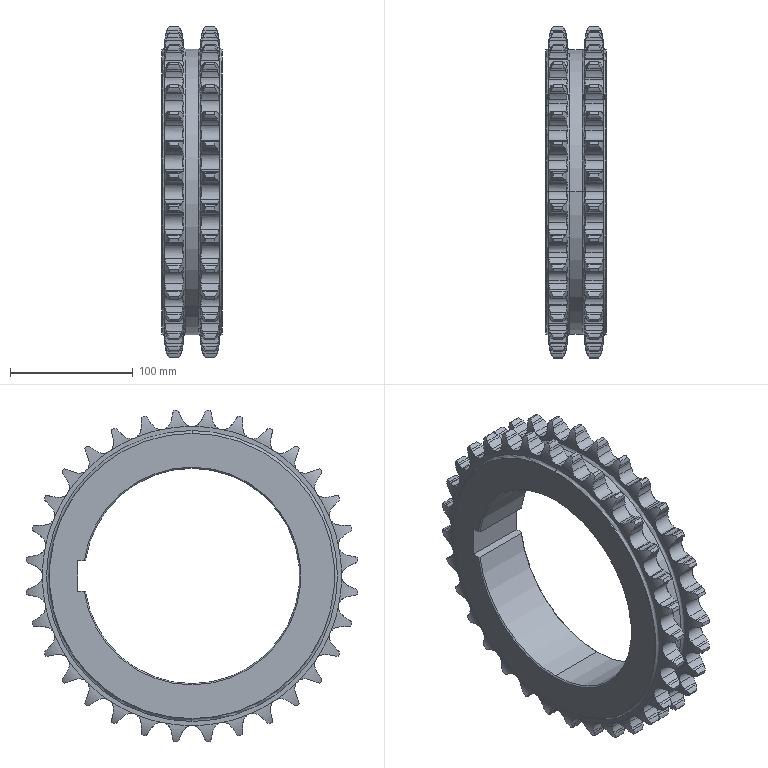Part | SolidWorks | features BaseBody 1 | 1 solid | 706 faces | box 49.567 x 269.954 x 269.954 mm | volume 1130107 mm3 | cylinder 427 | plane 137 | torus 136 | cone 6 | commonest cylinder face diameters 22.807 x136 41.467 x136 16.059 x82 271 x64 232 x6 175 x3